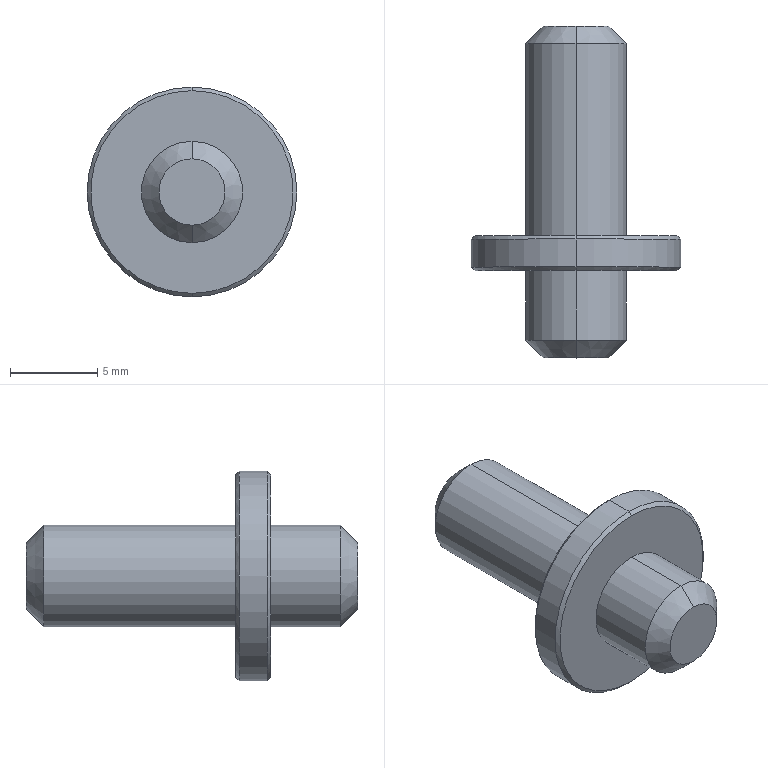Part | SolidWorks | features BaseBody 1 | 1 solid | 18 faces | box 12 x 19 x 12 mm | volume 657.73 mm3 | cone 8 | cylinder 6 | plane 4 | commonest cylinder face diameters 5.8 x4 12 x2
STEP:
#1=CARTESIAN_POINT('',(0.,2.,2.9));
#2=VERTEX_POINT('',#1);
#3=CARTESIAN_POINT('',(0.,2.,-2.9));
#4=VERTEX_POINT('',#3);
#5=CARTESIAN_POINT('',(0.,2.,0.));
#6=DIRECTION('',(0.,1.,0.));
#7=DIRECTION('',(0.,0.,1.));
#8=AXIS2_PLACEMENT_3D('',#5,#6,#7);
#9=CIRCLE('',#8,2.9);
#10=EDGE_CURVE('',#2,#4,#9,.T.);
#11=ORIENTED_EDGE('',*,*,#10,.T.);
#12=CARTESIAN_POINT('',(0.,13.,-2.9));
#13=VERTEX_POINT('',#12);
#14=CARTESIAN_POINT('',(0.,2.,-2.9));
#15=DIRECTION('',(0.,1.,0.));
#16=VECTOR('',#15,1000.);
#17=LINE('',#14,#16);
#18=EDGE_CURVE('',#4,#13,#17,.T.);
#19=ORIENTED_EDGE('',*,*,#18,.T.);
#20=CARTESIAN_POINT('',(0.,13.,2.9));
#21=VERTEX_POINT('',#20);
#22=CARTESIAN_POINT('',(0.,13.,0.));
#23=DIRECTION('',(0.,-1.,0.));
#24=DIRECTION('',(0.,0.,1.));
#25=AXIS2_PLACEMENT_3D('',#22,#23,#24);
#26=CIRCLE('',#25,2.9);
#27=EDGE_CURVE('',#13,#21,#26,.T.);
#28=ORIENTED_EDGE('',*,*,#27,.T.);
#29=CARTESIAN_POINT('',(0.,2.,2.9));
#30=DIRECTION('',(0.,1.,0.));
#31=VECTOR('',#30,1000.);
#32=LINE('',#29,#31);
#33=EDGE_CURVE('',#2,#21,#32,.T.);
#34=ORIENTED_EDGE('',*,*,#33,.F.);
#35=EDGE_LOOP('',(#11,#19,#28,#34));
#36=FACE_OUTER_BOUND('',#35,.T.);
#37=CARTESIAN_POINT('',(0.,2.,0.));
#38=DIRECTION('',(0.,1.,0.));
#39=DIRECTION('',(0.,0.,1.));
#40=AXIS2_PLACEMENT_3D('',#37,#38,#39);
#41=CYLINDRICAL_SURFACE('',#40,2.9);
#42=ADVANCED_FACE('',(#36),#41,.T.);
#43=CARTESIAN_POINT('',(0.,14.,-1.9));
#44=VERTEX_POINT('',#43);
#45=CARTESIAN_POINT('',(0.,14.,1.9));
#46=VERTEX_POINT('',#45);
#47=CARTESIAN_POINT('',(0.,14.,0.));
#48=DIRECTION('',(0.,-1.,0.));
#49=DIRECTION('',(0.,0.,-1.));
#50=AXIS2_PLACEMENT_3D('',#47,#48,#49);
#51=CIRCLE('',#50,1.9);
#52=EDGE_CURVE('',#44,#46,#51,.T.);
#53=ORIENTED_EDGE('',*,*,#52,.T.);
#54=CARTESIAN_POINT('',(0.,13.,2.9));
#55=DIRECTION('',(0.,-0.7071,0.7071));
#56=VECTOR('',#55,1000.);
#57=LINE('',#54,#56);
#58=EDGE_CURVE('',#46,#21,#57,.T.);
#59=ORIENTED_EDGE('',*,*,#58,.T.);
#60=ORIENTED_EDGE('',*,*,#27,.F.);
#61=CARTESIAN_POINT('',(0.,13.,-2.9));
#62=DIRECTION('',(0.,-0.7071,-0.7071));
#63=VECTOR('',#62,1000.);
#64=LINE('',#61,#63);
#65=EDGE_CURVE('',#44,#13,#64,.T.);
#66=ORIENTED_EDGE('',*,*,#65,.F.);
#67=EDGE_LOOP('',(#53,#59,#60,#66));
#68=FACE_OUTER_BOUND('',#67,.T.);
#69=CARTESIAN_POINT('',(0.,13.,0.));
#70=DIRECTION('',(0.,-1.,0.));
#71=DIRECTION('',(0.,0.,-1.));
#72=AXIS2_PLACEMENT_3D('',#69,#70,#71);
#73=CONICAL_SURFACE('',#72,2.9,0.7854);
#74=ADVANCED_FACE('',(#68),#73,.T.);
#75=CARTESIAN_POINT('',(0.,2.,5.8));
#76=VERTEX_POINT('',#75);
#77=CARTESIAN_POINT('',(0.,2.,-5.8));
#78=VERTEX_POINT('',#77);
#79=CARTESIAN_POINT('',(0.,2.,0.));
#80=DIRECTION('',(0.,1.,0.));
#81=DIRECTION('',(0.,0.,-1.));
#82=AXIS2_PLACEMENT_3D('',#79,#80,#81);
#83=CIRCLE('',#82,5.8);
#84=EDGE_CURVE('',#76,#78,#83,.T.);
#85=ORIENTED_EDGE('',*,*,#84,.F.);
#86=CARTESIAN_POINT('',(0.,1.8,6.));
#87=VERTEX_POINT('',#86);
#88=CARTESIAN_POINT('',(0.,1.8,6.));
#89=DIRECTION('',(0.,-0.7071,0.7071));
#90=VECTOR('',#89,1000.);
#91=LINE('',#88,#90);
#92=EDGE_CURVE('',#76,#87,#91,.T.);
#93=ORIENTED_EDGE('',*,*,#92,.T.);
#94=CARTESIAN_POINT('',(0.,1.8,-6.));
#95=VERTEX_POINT('',#94);
#96=CARTESIAN_POINT('',(0.,1.8,0.));
#97=DIRECTION('',(0.,1.,0.));
#98=DIRECTION('',(0.,0.,-1.));
#99=AXIS2_PLACEMENT_3D('',#96,#97,#98);
#100=CIRCLE('',#99,6.);
#101=EDGE_CURVE('',#87,#95,#100,.T.);
#102=ORIENTED_EDGE('',*,*,#101,.T.);
#103=CARTESIAN_POINT('',(0.,1.8,-6.));
#104=DIRECTION('',(0.,-0.7071,-0.7071));
#105=VECTOR('',#104,1000.);
#106=LINE('',#103,#105);
#107=EDGE_CURVE('',#78,#95,#106,.T.);
#108=ORIENTED_EDGE('',*,*,#107,.F.);
#109=EDGE_LOOP('',(#85,#93,#102,#108));
#110=FACE_OUTER_BOUND('',#109,.T.);
#111=CARTESIAN_POINT('',(0.,1.8,0.));
#112=DIRECTION('',(0.,-1.,0.));
#113=DIRECTION('',(0.,0.,-1.));
#114=AXIS2_PLACEMENT_3D('',#111,#112,#113);
#115=CONICAL_SURFACE('',#114,6.,0.7854);
#116=ADVANCED_FACE('',(#110),#115,.T.);
#117=CARTESIAN_POINT('',(0.,0.2,6.));
#118=VERTEX_POINT('',#117);
#119=CARTESIAN_POINT('',(0.,0.2,-6.));
#120=VERTEX_POINT('',#119);
#121=CARTESIAN_POINT('',(0.,0.2,0.));
#122=DIRECTION('',(0.,1.,0.));
#123=DIRECTION('',(0.,0.,1.));
#124=AXIS2_PLACEMENT_3D('',#121,#122,#123);
#125=CIRCLE('',#124,6.);
#126=EDGE_CURVE('',#118,#120,#125,.T.);
#127=ORIENTED_EDGE('',*,*,#126,.T.);
#128=CARTESIAN_POINT('',(0.,0.,-6.));
#129=DIRECTION('',(0.,1.,0.));
#130=VECTOR('',#129,1000.);
#131=LINE('',#128,#130);
#132=EDGE_CURVE('',#120,#95,#131,.T.);
#133=ORIENTED_EDGE('',*,*,#132,.T.);
#134=ORIENTED_EDGE('',*,*,#101,.F.);
#135=CARTESIAN_POINT('',(0.,0.,6.));
#136=DIRECTION('',(0.,1.,0.));
#137=VECTOR('',#136,1000.);
#138=LINE('',#135,#137);
#139=EDGE_CURVE('',#118,#87,#138,.T.);
#140=ORIENTED_EDGE('',*,*,#139,.F.);
#141=EDGE_LOOP('',(#127,#133,#134,#140));
#142=FACE_OUTER_BOUND('',#141,.T.);
#143=CARTESIAN_POINT('',(0.,0.,0.));
#144=DIRECTION('',(0.,1.,0.));
#145=DIRECTION('',(0.,0.,1.));
#146=AXIS2_PLACEMENT_3D('',#143,#144,#145);
#147=CYLINDRICAL_SURFACE('',#146,6.);
#148=ADVANCED_FACE('',(#142),#147,.T.);
#149=CARTESIAN_POINT('',(0.,0.,5.8));
#150=VERTEX_POINT('',#149);
#151=CARTESIAN_POINT('',(0.,0.,-5.8));
#152=VERTEX_POINT('',#151);
#153=CARTESIAN_POINT('',(0.,0.,0.));
#154=DIRECTION('',(0.,1.,0.));
#155=DIRECTION('',(0.,0.,1.));
#156=AXIS2_PLACEMENT_3D('',#153,#154,#155);
#157=CIRCLE('',#156,5.8);
#158=EDGE_CURVE('',#150,#152,#157,.T.);
#159=ORIENTED_EDGE('',*,*,#158,.T.);
#160=CARTESIAN_POINT('',(0.,0.2,-6.));
#161=DIRECTION('',(0.,0.7071,-0.7071));
#162=VECTOR('',#161,1000.);
#163=LINE('',#160,#162);
#164=EDGE_CURVE('',#152,#120,#163,.T.);
#165=ORIENTED_EDGE('',*,*,#164,.T.);
#166=ORIENTED_EDGE('',*,*,#126,.F.);
#167=CARTESIAN_POINT('',(0.,0.2,6.));
#168=DIRECTION('',(0.,0.7071,0.7071));
#169=VECTOR('',#168,1000.);
#170=LINE('',#167,#169);
#171=EDGE_CURVE('',#150,#118,#170,.T.);
#172=ORIENTED_EDGE('',*,*,#171,.F.);
#173=EDGE_LOOP('',(#159,#165,#166,#172));
#174=FACE_OUTER_BOUND('',#173,.T.);
#175=CARTESIAN_POINT('',(0.,0.2,0.));
#176=DIRECTION('',(0.,1.,0.));
#177=DIRECTION('',(0.,0.,1.));
#178=AXIS2_PLACEMENT_3D('',#175,#176,#177);
#179=CONICAL_SURFACE('',#178,6.,0.7854);
#180=ADVANCED_FACE('',(#174),#179,.T.);
#181=CARTESIAN_POINT('',(0.,0.,-2.9));
#182=VERTEX_POINT('',#181);
#183=CARTESIAN_POINT('',(0.,0.,2.9));
#184=VERTEX_POINT('',#183);
#185=CARTESIAN_POINT('',(0.,0.,0.));
#186=DIRECTION('',(0.,-1.,0.));
#187=DIRECTION('',(0.,0.,-1.));
#188=AXIS2_PLACEMENT_3D('',#185,#186,#187);
#189=CIRCLE('',#188,2.9);
#190=EDGE_CURVE('',#182,#184,#189,.T.);
#191=ORIENTED_EDGE('',*,*,#190,.T.);
#192=CARTESIAN_POINT('',(0.,-4.,2.9));
#193=VERTEX_POINT('',#192);
#194=CARTESIAN_POINT('',(0.,0.,2.9));
#195=DIRECTION('',(0.,-1.,0.));
#196=VECTOR('',#195,1000.);
#197=LINE('',#194,#196);
#198=EDGE_CURVE('',#184,#193,#197,.T.);
#199=ORIENTED_EDGE('',*,*,#198,.T.);
#200=CARTESIAN_POINT('',(0.,-4.,-2.9));
#201=VERTEX_POINT('',#200);
#202=CARTESIAN_POINT('',(0.,-4.,0.));
#203=DIRECTION('',(0.,1.,0.));
#204=DIRECTION('',(0.,0.,-1.));
#205=AXIS2_PLACEMENT_3D('',#202,#203,#204);
#206=CIRCLE('',#205,2.9);
#207=EDGE_CURVE('',#193,#201,#206,.T.);
#208=ORIENTED_EDGE('',*,*,#207,.T.);
#209=CARTESIAN_POINT('',(0.,0.,-2.9));
#210=DIRECTION('',(0.,-1.,0.));
#211=VECTOR('',#210,1000.);
#212=LINE('',#209,#211);
#213=EDGE_CURVE('',#182,#201,#212,.T.);
#214=ORIENTED_EDGE('',*,*,#213,.F.);
#215=EDGE_LOOP('',(#191,#199,#208,#214));
#216=FACE_OUTER_BOUND('',#215,.T.);
#217=CARTESIAN_POINT('',(0.,0.,0.));
#218=DIRECTION('',(0.,-1.,0.));
#219=DIRECTION('',(0.,0.,-1.));
#220=AXIS2_PLACEMENT_3D('',#217,#218,#219);
#221=CYLINDRICAL_SURFACE('',#220,2.9);
#222=ADVANCED_FACE('',(#216),#221,.T.);
#223=CARTESIAN_POINT('',(0.,-5.,1.9));
#224=VERTEX_POINT('',#223);
#225=CARTESIAN_POINT('',(0.,-5.,-1.9));
#226=VERTEX_POINT('',#225);
#227=CARTESIAN_POINT('',(0.,-5.,0.));
#228=DIRECTION('',(0.,1.,0.));
#229=DIRECTION('',(0.,0.,1.));
#230=AXIS2_PLACEMENT_3D('',#227,#228,#229);
#231=CIRCLE('',#230,1.9);
#232=EDGE_CURVE('',#224,#226,#231,.T.);
#233=ORIENTED_EDGE('',*,*,#232,.T.);
#234=CARTESIAN_POINT('',(0.,-4.,-2.9));
#235=DIRECTION('',(0.,0.7071,-0.7071));
#236=VECTOR('',#235,1000.);
#237=LINE('',#234,#236);
#238=EDGE_CURVE('',#226,#201,#237,.T.);
#239=ORIENTED_EDGE('',*,*,#238,.T.);
#240=ORIENTED_EDGE('',*,*,#207,.F.);
#241=CARTESIAN_POINT('',(0.,-4.,2.9));
#242=DIRECTION('',(0.,0.7071,0.7071));
#243=VECTOR('',#242,1000.);
#244=LINE('',#241,#243);
#245=EDGE_CURVE('',#224,#193,#244,.T.);
#246=ORIENTED_EDGE('',*,*,#245,.F.);
#247=EDGE_LOOP('',(#233,#239,#240,#246));
#248=FACE_OUTER_BOUND('',#247,.T.);
#249=CARTESIAN_POINT('',(0.,-4.,0.));
#250=DIRECTION('',(0.,1.,0.));
#251=DIRECTION('',(0.,0.,1.));
#252=AXIS2_PLACEMENT_3D('',#249,#250,#251);
#253=CONICAL_SURFACE('',#252,2.9,0.7854);
#254=ADVANCED_FACE('',(#248),#253,.T.);
#255=ORIENTED_EDGE('',*,*,#18,.F.);
#256=CARTESIAN_POINT('',(0.,2.,0.));
#257=DIRECTION('',(0.,1.,0.));
#258=DIRECTION('',(0.,0.,1.));
#259=AXIS2_PLACEMENT_3D('',#256,#257,#258);
#260=CIRCLE('',#259,2.9);
#261=EDGE_CURVE('',#4,#2,#260,.T.);
#262=ORIENTED_EDGE('',*,*,#261,.T.);
#263=ORIENTED_EDGE('',*,*,#33,.T.);
#264=CARTESIAN_POINT('',(0.,13.,0.));
#265=DIRECTION('',(0.,-1.,0.));
#266=DIRECTION('',(0.,0.,1.));
#267=AXIS2_PLACEMENT_3D('',#264,#265,#266);
#268=CIRCLE('',#267,2.9);
#269=EDGE_CURVE('',#21,#13,#268,.T.);
#270=ORIENTED_EDGE('',*,*,#269,.T.);
#271=EDGE_LOOP('',(#255,#262,#263,#270));
#272=FACE_OUTER_BOUND('',#271,.T.);
#273=CARTESIAN_POINT('',(0.,2.,0.));
#274=DIRECTION('',(0.,1.,0.));
#275=DIRECTION('',(0.,0.,1.));
#276=AXIS2_PLACEMENT_3D('',#273,#274,#275);
#277=CYLINDRICAL_SURFACE('',#276,2.9);
#278=ADVANCED_FACE('',(#272),#277,.T.);
#279=ORIENTED_EDGE('',*,*,#58,.F.);
#280=CARTESIAN_POINT('',(0.,14.,0.));
#281=DIRECTION('',(0.,-1.,0.));
#282=DIRECTION('',(0.,0.,-1.));
#283=AXIS2_PLACEMENT_3D('',#280,#281,#282);
#284=CIRCLE('',#283,1.9);
#285=EDGE_CURVE('',#46,#44,#284,.T.);
#286=ORIENTED_EDGE('',*,*,#285,.T.);
#287=ORIENTED_EDGE('',*,*,#65,.T.);
#288=ORIENTED_EDGE('',*,*,#269,.F.);
#289=EDGE_LOOP('',(#279,#286,#287,#288));
#290=FACE_OUTER_BOUND('',#289,.T.);
#291=CARTESIAN_POINT('',(0.,13.,0.));
#292=DIRECTION('',(0.,-1.,0.));
#293=DIRECTION('',(0.,0.,-1.));
#294=AXIS2_PLACEMENT_3D('',#291,#292,#293);
#295=CONICAL_SURFACE('',#294,2.9,0.7854);
#296=ADVANCED_FACE('',(#290),#295,.T.);
#297=ORIENTED_EDGE('',*,*,#10,.F.);
#298=ORIENTED_EDGE('',*,*,#261,.F.);
#299=EDGE_LOOP('',(#297,#298));
#300=FACE_BOUND('',#299,.T.);
#301=CARTESIAN_POINT('',(0.,2.,0.));
#302=DIRECTION('',(0.,1.,0.));
#303=DIRECTION('',(0.,0.,-1.));
#304=AXIS2_PLACEMENT_3D('',#301,#302,#303);
#305=CIRCLE('',#304,5.8);
#306=EDGE_CURVE('',#78,#76,#305,.T.);
#307=ORIENTED_EDGE('',*,*,#306,.T.);
#308=ORIENTED_EDGE('',*,*,#84,.T.);
#309=EDGE_LOOP('',(#307,#308));
#310=FACE_OUTER_BOUND('',#309,.T.);
#311=CARTESIAN_POINT('',(0.,2.,0.));
#312=DIRECTION('',(0.,1.,0.));
#313=DIRECTION('',(0.,0.,1.));
#314=AXIS2_PLACEMENT_3D('',#311,#312,#313);
#315=PLANE('',#314);
#316=ADVANCED_FACE('',(#300,#310),#315,.T.);
#317=ORIENTED_EDGE('',*,*,#52,.F.);
#318=ORIENTED_EDGE('',*,*,#285,.F.);
#319=EDGE_LOOP('',(#317,#318));
#320=FACE_OUTER_BOUND('',#319,.T.);
#321=CARTESIAN_POINT('',(0.,14.,0.));
#322=DIRECTION('',(0.,1.,0.));
#323=DIRECTION('',(0.,0.,1.));
#324=AXIS2_PLACEMENT_3D('',#321,#322,#323);
#325=PLANE('',#324);
#326=ADVANCED_FACE('',(#320),#325,.T.);
#327=ORIENTED_EDGE('',*,*,#92,.F.);
#328=ORIENTED_EDGE('',*,*,#306,.F.);
#329=ORIENTED_EDGE('',*,*,#107,.T.);
#330=CARTESIAN_POINT('',(0.,1.8,0.));
#331=DIRECTION('',(0.,1.,0.));
#332=DIRECTION('',(0.,0.,-1.));
#333=AXIS2_PLACEMENT_3D('',#330,#331,#332);
#334=CIRCLE('',#333,6.);
#335=EDGE_CURVE('',#95,#87,#334,.T.);
#336=ORIENTED_EDGE('',*,*,#335,.T.);
#337=EDGE_LOOP('',(#327,#328,#329,#336));
#338=FACE_OUTER_BOUND('',#337,.T.);
#339=CARTESIAN_POINT('',(0.,1.8,0.));
#340=DIRECTION('',(0.,-1.,0.));
#341=DIRECTION('',(0.,0.,-1.));
#342=AXIS2_PLACEMENT_3D('',#339,#340,#341);
#343=CONICAL_SURFACE('',#342,6.,0.7854);
#344=ADVANCED_FACE('',(#338),#343,.T.);
#345=ORIENTED_EDGE('',*,*,#132,.F.);
#346=CARTESIAN_POINT('',(0.,0.2,0.));
#347=DIRECTION('',(0.,1.,0.));
#348=DIRECTION('',(0.,0.,1.));
#349=AXIS2_PLACEMENT_3D('',#346,#347,#348);
#350=CIRCLE('',#349,6.);
#351=EDGE_CURVE('',#120,#118,#350,.T.);
#352=ORIENTED_EDGE('',*,*,#351,.T.);
#353=ORIENTED_EDGE('',*,*,#139,.T.);
#354=ORIENTED_EDGE('',*,*,#335,.F.);
#355=EDGE_LOOP('',(#345,#352,#353,#354));
#356=FACE_OUTER_BOUND('',#355,.T.);
#357=CARTESIAN_POINT('',(0.,0.,0.));
#358=DIRECTION('',(0.,1.,0.));
#359=DIRECTION('',(0.,0.,1.));
#360=AXIS2_PLACEMENT_3D('',#357,#358,#359);
#361=CYLINDRICAL_SURFACE('',#360,6.);
#362=ADVANCED_FACE('',(#356),#361,.T.);
#363=ORIENTED_EDGE('',*,*,#164,.F.);
#364=CARTESIAN_POINT('',(0.,0.,0.));
#365=DIRECTION('',(0.,1.,0.));
#366=DIRECTION('',(0.,0.,1.));
#367=AXIS2_PLACEMENT_3D('',#364,#365,#366);
#368=CIRCLE('',#367,5.8);
#369=EDGE_CURVE('',#152,#150,#368,.T.);
#370=ORIENTED_EDGE('',*,*,#369,.T.);
#371=ORIENTED_EDGE('',*,*,#171,.T.);
#372=ORIENTED_EDGE('',*,*,#351,.F.);
#373=EDGE_LOOP('',(#363,#370,#371,#372));
#374=FACE_OUTER_BOUND('',#373,.T.);
#375=CARTESIAN_POINT('',(0.,0.2,0.));
#376=DIRECTION('',(0.,1.,0.));
#377=DIRECTION('',(0.,0.,1.));
#378=AXIS2_PLACEMENT_3D('',#375,#376,#377);
#379=CONICAL_SURFACE('',#378,6.,0.7854);
#380=ADVANCED_FACE('',(#374),#379,.T.);
#381=ORIENTED_EDGE('',*,*,#190,.F.);
#382=CARTESIAN_POINT('',(0.,0.,0.));
#383=DIRECTION('',(0.,-1.,0.));
#384=DIRECTION('',(0.,0.,-1.));
#385=AXIS2_PLACEMENT_3D('',#382,#383,#384);
#386=CIRCLE('',#385,2.9);
#387=EDGE_CURVE('',#184,#182,#386,.T.);
#388=ORIENTED_EDGE('',*,*,#387,.F.);
#389=EDGE_LOOP('',(#381,#388));
#390=FACE_BOUND('',#389,.T.);
#391=ORIENTED_EDGE('',*,*,#158,.F.);
#392=ORIENTED_EDGE('',*,*,#369,.F.);
#393=EDGE_LOOP('',(#391,#392));
#394=FACE_OUTER_BOUND('',#393,.T.);
#395=CARTESIAN_POINT('',(0.,0.,0.));
#396=DIRECTION('',(0.,1.,0.));
#397=DIRECTION('',(0.,0.,1.));
#398=AXIS2_PLACEMENT_3D('',#395,#396,#397);
#399=PLANE('',#398);
#400=ADVANCED_FACE('',(#390,#394),#399,.F.);
#401=ORIENTED_EDGE('',*,*,#198,.F.);
#402=ORIENTED_EDGE('',*,*,#387,.T.);
#403=ORIENTED_EDGE('',*,*,#213,.T.);
#404=CARTESIAN_POINT('',(0.,-4.,0.));
#405=DIRECTION('',(0.,1.,0.));
#406=DIRECTION('',(0.,0.,-1.));
#407=AXIS2_PLACEMENT_3D('',#404,#405,#406);
#408=CIRCLE('',#407,2.9);
#409=EDGE_CURVE('',#201,#193,#408,.T.);
#410=ORIENTED_EDGE('',*,*,#409,.T.);
#411=EDGE_LOOP('',(#401,#402,#403,#410));
#412=FACE_OUTER_BOUND('',#411,.T.);
#413=CARTESIAN_POINT('',(0.,0.,0.));
#414=DIRECTION('',(0.,-1.,0.));
#415=DIRECTION('',(0.,0.,-1.));
#416=AXIS2_PLACEMENT_3D('',#413,#414,#415);
#417=CYLINDRICAL_SURFACE('',#416,2.9);
#418=ADVANCED_FACE('',(#412),#417,.T.);
#419=ORIENTED_EDGE('',*,*,#238,.F.);
#420=CARTESIAN_POINT('',(0.,-5.,0.));
#421=DIRECTION('',(0.,1.,0.));
#422=DIRECTION('',(0.,0.,1.));
#423=AXIS2_PLACEMENT_3D('',#420,#421,#422);
#424=CIRCLE('',#423,1.9);
#425=EDGE_CURVE('',#226,#224,#424,.T.);
#426=ORIENTED_EDGE('',*,*,#425,.T.);
#427=ORIENTED_EDGE('',*,*,#245,.T.);
#428=ORIENTED_EDGE('',*,*,#409,.F.);
#429=EDGE_LOOP('',(#419,#426,#427,#428));
#430=FACE_OUTER_BOUND('',#429,.T.);
#431=CARTESIAN_POINT('',(0.,-4.,0.));
#432=DIRECTION('',(0.,1.,0.));
#433=DIRECTION('',(0.,0.,1.));
#434=AXIS2_PLACEMENT_3D('',#431,#432,#433);
#435=CONICAL_SURFACE('',#434,2.9,0.7854);
#436=ADVANCED_FACE('',(#430),#435,.T.);
#437=ORIENTED_EDGE('',*,*,#232,.F.);
#438=ORIENTED_EDGE('',*,*,#425,.F.);
#439=EDGE_LOOP('',(#437,#438));
#440=FACE_OUTER_BOUND('',#439,.T.);
#441=CARTESIAN_POINT('',(0.,-5.,0.));
#442=DIRECTION('',(0.,-1.,0.));
#443=DIRECTION('',(0.,0.,-1.));
#444=AXIS2_PLACEMENT_3D('',#441,#442,#443);
#445=PLANE('',#444);
#446=ADVANCED_FACE('',(#440),#445,.T.);
#447=CLOSED_SHELL('',(#42,#74,#116,#148,#180,#222,#254,#278,#296,#316,#326,#344,#362,#380,#400,#418,#436,#446));
#448=MANIFOLD_SOLID_BREP('',#447);
#449=CARTESIAN_POINT('',(0.,0.,0.));
#450=DIRECTION('',(0.,0.,1.));
#451=DIRECTION('',(1.,0.,0.));
#452=AXIS2_PLACEMENT_3D('',#449,#450,#451);
#453=(LENGTH_UNIT()NAMED_UNIT(*)SI_UNIT(.MILLI.,.METRE.));
#454=UNCERTAINTY_MEASURE_WITH_UNIT(LENGTH_MEASURE(0.00001),#453,'','');
#455=(NAMED_UNIT(*)PLANE_ANGLE_UNIT()SI_UNIT($,.RADIAN.));
#456=(NAMED_UNIT(*)SI_UNIT($,.STERADIAN.)SOLID_ANGLE_UNIT());
#457=(GEOMETRIC_REPRESENTATION_CONTEXT(3)GLOBAL_UNCERTAINTY_ASSIGNED_CONTEXT((#454))GLOBAL_UNIT_ASSIGNED_CONTEXT((#453,#455,#456))REPRESENTATION_CONTEXT('',''));
#458=ADVANCED_BREP_SHAPE_REPRESENTATION('',(#448,#452),#457);